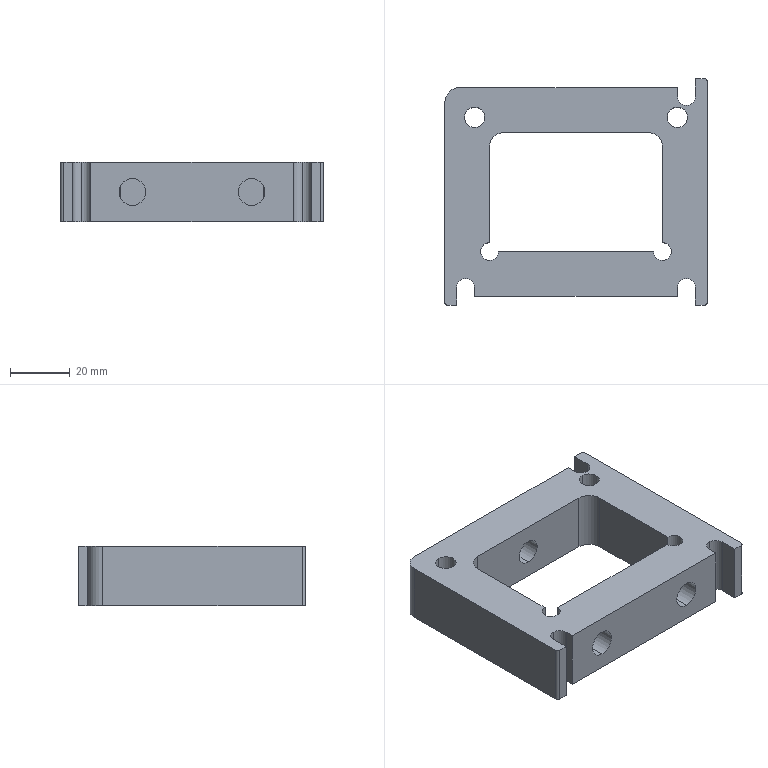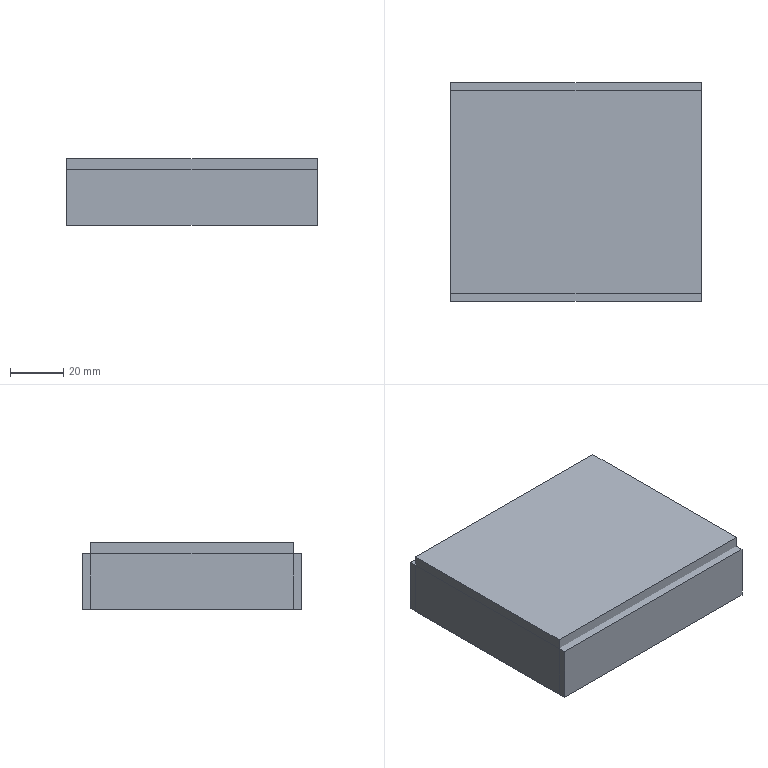CAM job | NX | 3-axis milling, drilling | part box 88 x 76 x 20 mm | stock box 94 x 82 x 25 mm
Tools:
number,name,description,diameter,corner_radius,flute_length,length,flutes
1,D63,Milling Tool-5 Parameters,63.0,0.0,50.0,75.0,2
7,D6A45,Milling Tool-5 Parameters,6.0,0.0,3.0,3.0,2
16,6.8ZT,Drilling Tool,6.8,0.0,35.0,50.0,2
17,6.0ZT,Drilling Tool,6.0,0.0,35.0,50.0,2
10,D10,Milling Tool-5 Parameters,10.0,0.0,50.0,75.0,2
11,D10JING,Milling Tool-5 Parameters,10.0,0.0,50.0,75.0,2
4,D4,Milling Tool-5 Parameters,4.0,0.0,50.0,75.0,2
Operations:
program,operation,operation_type,tool,method,geometry_group,spindle_rpm,surface_speed,feed_per_tooth,feed_cut,feed_plunge,cut_length_mm,path_length_mm,cut_time_min,machine_time_min
1-80-90-25毛胚,FLOOR_WALL,VolumeBased25DMillingOperation,D63,METHOD,A,6500.0,1286.0,0.0962,1250.0,100.0,539.797,593.797,0.4318,0.4372
1-80-90-25毛胚,DRILLING_COPY_1,Operation,D6A45,METHOD,A,3000.0,56.0,0.0333,200.0,0.0,24.0,311.28,0.12,0.1487
1-80-90-25毛胚,DRILLING_COPY_1_COPY,Operation,6.8ZT,METHOD,A,2000.0,42.0,0.05,200.0,0.0,53.086,237.238,0.2654,0.2838
1-80-90-25毛胚,DRILLING_COPY_1_COPY_COPY,Operation,6.0ZT,METHOD,A,2000.0,42.0,0.05,200.0,0.0,52.605,226.288,0.263,0.2804
1-80-90-25毛胚,ADAPTIVE_MILLING,CavityMilling,D10,METHOD,A,8000.0,251.0,0.2188,3500.0,1000.0,6717.114,6949.964,2.863,2.886
1-80-90-25毛胚,ZLEVEL_PROFILE_COPY_COPY_1,ZLevelMilling,D10JING,METHOD,A,8000.0,251.0,0.05,800.0,100.0,525.195,758.132,0.6565,0.6798
1-80-90-25毛胚,ZLEVEL_PROFILE_COPY_1_COPY_1_COPY_1_1_COPY_COPY,ZLevelMilling,D4,METHOD,A,8000.0,100.0,0.0875,1400.0,800.0,5562.325,7653.126,4.173,4.382
1-80-90-25毛胚,ZLEVEL_PROFILE_1_COPY_1_COPY_COPY_1_COPY,ZLevelMilling,D6A45,METHOD,A,7500.0,141.0,0.0667,1000.0,100.0,612.161,940.784,0.6122,0.645
2-80-90-25毛胚,FLOOR_WALL_COPY,VolumeBased25DMillingOperation,D63,METHOD,B,6500.0,1286.0,0.0962,1250.0,100.0,2668.985,3601.913,2.135,2.228
2-80-90-25毛胚,ZLEVEL_PROFILE_1_COPY_1_COPY_COPY_1_COPY_COPY,ZLevelMilling,D6A45,METHOD,B,7500.0,141.0,0.0667,1000.0,100.0,612.089,990.666,0.6121,0.6499